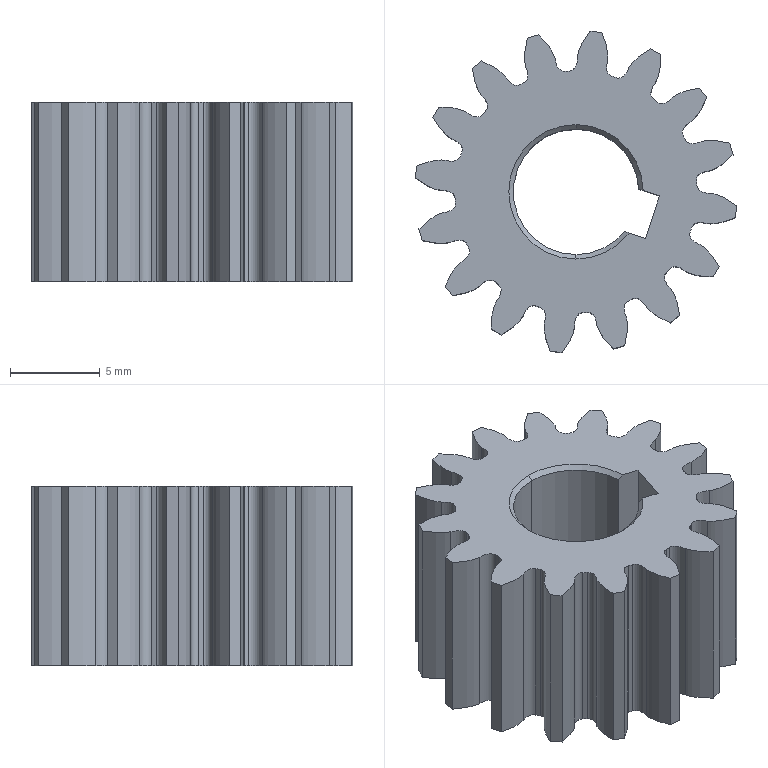Part | STEP file | GEAR_1_BODY-5 | 1 solid | 110 faces | box 17.933 x 17.933 x 10 mm | volume 1551 mm3 | spline 80 | cylinder 19 | cone 6 | plane 5 | commonest cylinder face diameters 13.5 x16 7 x3